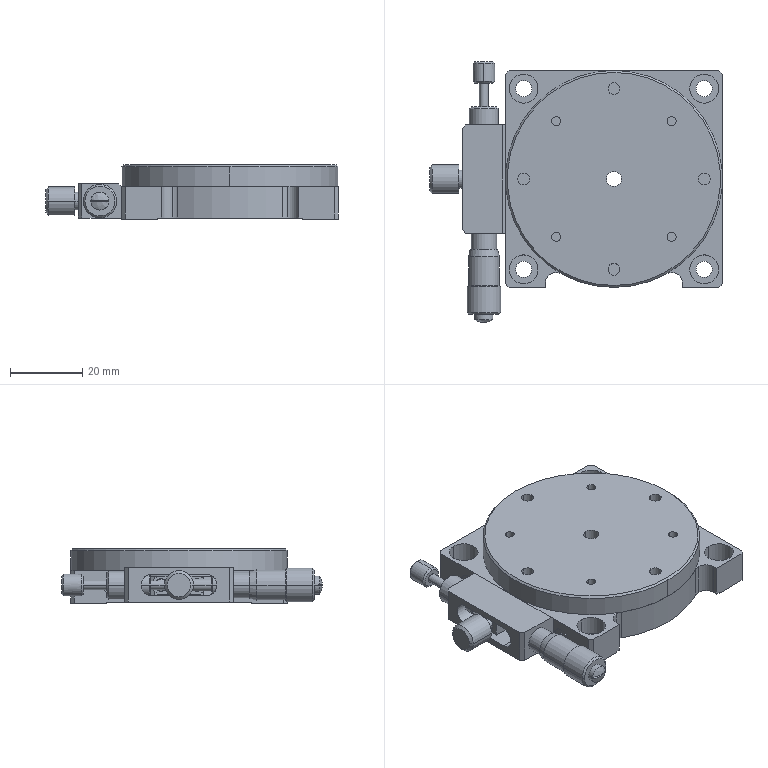Part | SolidWorks | 4 solids | 438 faces | box 81 x 72.197 x 15 mm | volume 47712 mm3 | plane 184 | cylinder 154 | cone 80 | spline 20 | commonest cylinder face diameters 6 x25 2.5 x14 3.5 x12 8 x12 3.3 x8 4.5 x8